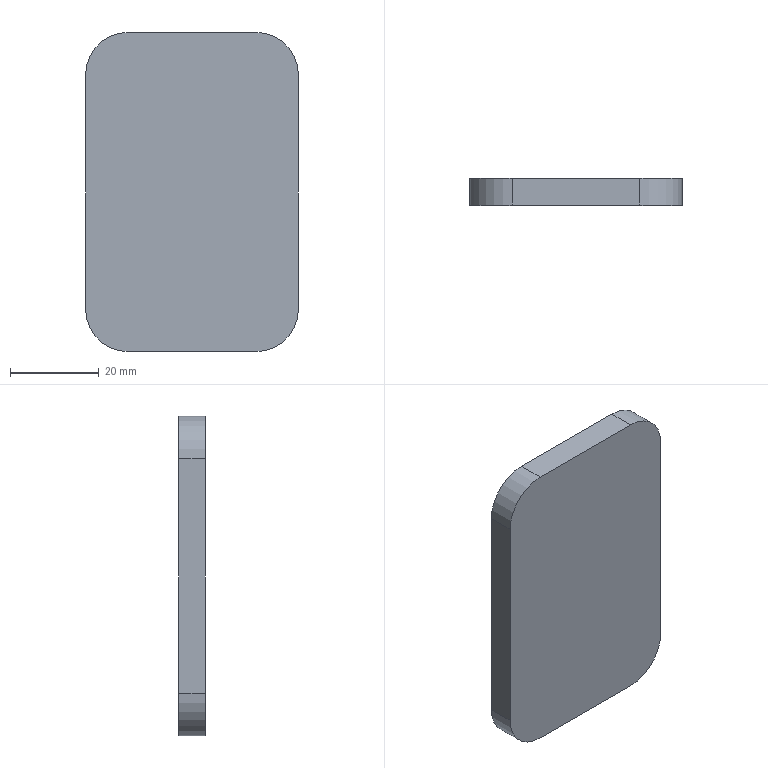Part | NX | 1 solid | 10 faces | box 48 x 6 x 72 mm | volume 20261 mm3 | plane 6 | cylinder 4 | commonest cylinder face diameters 19.2 x4
STEP:
#1=CARTESIAN_POINT('',(-7.326,-756.819,634.353));
#2=VERTEX_POINT('',#1);
#3=CARTESIAN_POINT('',(-16.926,-756.819,643.953));
#4=VERTEX_POINT('',#3);
#5=CARTESIAN_POINT('',(-16.926,-756.819,634.353));
#6=DIRECTION('',(0.,-1.,0.));
#7=DIRECTION('',(0.,0.,-1.));
#8=AXIS2_PLACEMENT_3D('',#5,#6,#7);
#9=CIRCLE('',#8,9.6);
#10=EDGE_CURVE('',#2,#4,#9,.T.);
#11=ORIENTED_EDGE('',*,*,#10,.T.);
#12=CARTESIAN_POINT('',(-16.926,-762.819,643.953));
#13=VERTEX_POINT('',#12);
#14=CARTESIAN_POINT('',(-16.926,-762.819,643.953));
#15=DIRECTION('',(0.,1.,0.));
#16=VECTOR('',#15,1.);
#17=LINE('',#14,#16);
#18=EDGE_CURVE('',#13,#4,#17,.T.);
#19=ORIENTED_EDGE('',*,*,#18,.F.);
#20=CARTESIAN_POINT('',(-7.326,-762.819,634.353));
#21=VERTEX_POINT('',#20);
#22=CARTESIAN_POINT('',(-16.926,-762.819,634.353));
#23=DIRECTION('',(0.,-1.,0.));
#24=DIRECTION('',(0.,0.,-1.));
#25=AXIS2_PLACEMENT_3D('',#22,#23,#24);
#26=CIRCLE('',#25,9.6);
#27=EDGE_CURVE('',#21,#13,#26,.T.);
#28=ORIENTED_EDGE('',*,*,#27,.F.);
#29=CARTESIAN_POINT('',(-7.326,-762.819,634.353));
#30=DIRECTION('',(0.,1.,0.));
#31=VECTOR('',#30,1.);
#32=LINE('',#29,#31);
#33=EDGE_CURVE('',#21,#2,#32,.T.);
#34=ORIENTED_EDGE('',*,*,#33,.T.);
#35=EDGE_LOOP('',(#11,#19,#28,#34));
#36=FACE_OUTER_BOUND('',#35,.T.);
#37=CARTESIAN_POINT('',(-16.926,-762.819,634.353));
#38=DIRECTION('',(0.,1.,0.));
#39=DIRECTION('',(0.,0.,1.));
#40=AXIS2_PLACEMENT_3D('',#37,#38,#39);
#41=CYLINDRICAL_SURFACE('',#40,9.6);
#42=ADVANCED_FACE('',(#36),#41,.T.);
#43=CARTESIAN_POINT('',(-45.726,-756.819,643.953));
#44=VERTEX_POINT('',#43);
#45=CARTESIAN_POINT('',(-16.926,-756.819,643.953));
#46=DIRECTION('',(-1.,0.,0.));
#47=VECTOR('',#46,1.);
#48=LINE('',#45,#47);
#49=EDGE_CURVE('',#4,#44,#48,.T.);
#50=ORIENTED_EDGE('',*,*,#49,.T.);
#51=CARTESIAN_POINT('',(-45.726,-762.819,643.953));
#52=VERTEX_POINT('',#51);
#53=CARTESIAN_POINT('',(-45.726,-762.819,643.953));
#54=DIRECTION('',(0.,1.,0.));
#55=VECTOR('',#54,1.);
#56=LINE('',#53,#55);
#57=EDGE_CURVE('',#52,#44,#56,.T.);
#58=ORIENTED_EDGE('',*,*,#57,.F.);
#59=CARTESIAN_POINT('',(-16.926,-762.819,643.953));
#60=DIRECTION('',(-1.,0.,0.));
#61=VECTOR('',#60,1.);
#62=LINE('',#59,#61);
#63=EDGE_CURVE('',#13,#52,#62,.T.);
#64=ORIENTED_EDGE('',*,*,#63,.F.);
#65=ORIENTED_EDGE('',*,*,#18,.T.);
#66=EDGE_LOOP('',(#50,#58,#64,#65));
#67=FACE_OUTER_BOUND('',#66,.T.);
#68=CARTESIAN_POINT('',(-16.926,-762.819,643.953));
#69=DIRECTION('',(0.,0.,-1.));
#70=DIRECTION('',(-1.,0.,0.));
#71=AXIS2_PLACEMENT_3D('',#68,#69,#70);
#72=PLANE('',#71);
#73=ADVANCED_FACE('',(#67),#72,.F.);
#74=CARTESIAN_POINT('',(-55.326,-756.819,634.353));
#75=VERTEX_POINT('',#74);
#76=CARTESIAN_POINT('',(-45.726,-756.819,634.353));
#77=DIRECTION('',(0.,-1.,0.));
#78=DIRECTION('',(0.,0.,-1.));
#79=AXIS2_PLACEMENT_3D('',#76,#77,#78);
#80=CIRCLE('',#79,9.6);
#81=EDGE_CURVE('',#44,#75,#80,.T.);
#82=ORIENTED_EDGE('',*,*,#81,.T.);
#83=CARTESIAN_POINT('',(-55.326,-762.819,634.353));
#84=VERTEX_POINT('',#83);
#85=CARTESIAN_POINT('',(-55.326,-762.819,634.353));
#86=DIRECTION('',(0.,1.,0.));
#87=VECTOR('',#86,1.);
#88=LINE('',#85,#87);
#89=EDGE_CURVE('',#84,#75,#88,.T.);
#90=ORIENTED_EDGE('',*,*,#89,.F.);
#91=CARTESIAN_POINT('',(-45.726,-762.819,634.353));
#92=DIRECTION('',(0.,-1.,0.));
#93=DIRECTION('',(0.,0.,-1.));
#94=AXIS2_PLACEMENT_3D('',#91,#92,#93);
#95=CIRCLE('',#94,9.6);
#96=EDGE_CURVE('',#52,#84,#95,.T.);
#97=ORIENTED_EDGE('',*,*,#96,.F.);
#98=ORIENTED_EDGE('',*,*,#57,.T.);
#99=EDGE_LOOP('',(#82,#90,#97,#98));
#100=FACE_OUTER_BOUND('',#99,.T.);
#101=CARTESIAN_POINT('',(-45.726,-762.819,634.353));
#102=DIRECTION('',(0.,1.,0.));
#103=DIRECTION('',(0.,0.,1.));
#104=AXIS2_PLACEMENT_3D('',#101,#102,#103);
#105=CYLINDRICAL_SURFACE('',#104,9.6);
#106=ADVANCED_FACE('',(#100),#105,.T.);
#107=CARTESIAN_POINT('',(-55.326,-756.819,581.553));
#108=VERTEX_POINT('',#107);
#109=CARTESIAN_POINT('',(-55.326,-756.819,634.353));
#110=DIRECTION('',(0.,0.,-1.));
#111=VECTOR('',#110,1.);
#112=LINE('',#109,#111);
#113=EDGE_CURVE('',#75,#108,#112,.T.);
#114=ORIENTED_EDGE('',*,*,#113,.T.);
#115=CARTESIAN_POINT('',(-55.326,-762.819,581.553));
#116=VERTEX_POINT('',#115);
#117=CARTESIAN_POINT('',(-55.326,-762.819,581.553));
#118=DIRECTION('',(0.,1.,0.));
#119=VECTOR('',#118,1.);
#120=LINE('',#117,#119);
#121=EDGE_CURVE('',#116,#108,#120,.T.);
#122=ORIENTED_EDGE('',*,*,#121,.F.);
#123=CARTESIAN_POINT('',(-55.326,-762.819,634.353));
#124=DIRECTION('',(0.,0.,-1.));
#125=VECTOR('',#124,1.);
#126=LINE('',#123,#125);
#127=EDGE_CURVE('',#84,#116,#126,.T.);
#128=ORIENTED_EDGE('',*,*,#127,.F.);
#129=ORIENTED_EDGE('',*,*,#89,.T.);
#130=EDGE_LOOP('',(#114,#122,#128,#129));
#131=FACE_OUTER_BOUND('',#130,.T.);
#132=CARTESIAN_POINT('',(-55.326,-762.819,634.353));
#133=DIRECTION('',(1.,0.,0.));
#134=DIRECTION('',(0.,0.,-1.));
#135=AXIS2_PLACEMENT_3D('',#132,#133,#134);
#136=PLANE('',#135);
#137=ADVANCED_FACE('',(#131),#136,.F.);
#138=CARTESIAN_POINT('',(-45.726,-756.819,571.953));
#139=VERTEX_POINT('',#138);
#140=CARTESIAN_POINT('',(-45.726,-756.819,581.553));
#141=DIRECTION('',(0.,-1.,0.));
#142=DIRECTION('',(0.,0.,-1.));
#143=AXIS2_PLACEMENT_3D('',#140,#141,#142);
#144=CIRCLE('',#143,9.6);
#145=EDGE_CURVE('',#108,#139,#144,.T.);
#146=ORIENTED_EDGE('',*,*,#145,.T.);
#147=CARTESIAN_POINT('',(-45.726,-762.819,571.953));
#148=VERTEX_POINT('',#147);
#149=CARTESIAN_POINT('',(-45.726,-762.819,571.953));
#150=DIRECTION('',(0.,1.,0.));
#151=VECTOR('',#150,1.);
#152=LINE('',#149,#151);
#153=EDGE_CURVE('',#148,#139,#152,.T.);
#154=ORIENTED_EDGE('',*,*,#153,.F.);
#155=CARTESIAN_POINT('',(-45.726,-762.819,581.553));
#156=DIRECTION('',(0.,-1.,0.));
#157=DIRECTION('',(0.,0.,-1.));
#158=AXIS2_PLACEMENT_3D('',#155,#156,#157);
#159=CIRCLE('',#158,9.6);
#160=EDGE_CURVE('',#116,#148,#159,.T.);
#161=ORIENTED_EDGE('',*,*,#160,.F.);
#162=ORIENTED_EDGE('',*,*,#121,.T.);
#163=EDGE_LOOP('',(#146,#154,#161,#162));
#164=FACE_OUTER_BOUND('',#163,.T.);
#165=CARTESIAN_POINT('',(-45.726,-762.819,581.553));
#166=DIRECTION('',(0.,1.,0.));
#167=DIRECTION('',(0.,0.,1.));
#168=AXIS2_PLACEMENT_3D('',#165,#166,#167);
#169=CYLINDRICAL_SURFACE('',#168,9.6);
#170=ADVANCED_FACE('',(#164),#169,.T.);
#171=CARTESIAN_POINT('',(-16.926,-756.819,571.953));
#172=VERTEX_POINT('',#171);
#173=CARTESIAN_POINT('',(-45.726,-756.819,571.953));
#174=DIRECTION('',(1.,0.,0.));
#175=VECTOR('',#174,1.);
#176=LINE('',#173,#175);
#177=EDGE_CURVE('',#139,#172,#176,.T.);
#178=ORIENTED_EDGE('',*,*,#177,.T.);
#179=CARTESIAN_POINT('',(-16.926,-762.819,571.953));
#180=VERTEX_POINT('',#179);
#181=CARTESIAN_POINT('',(-16.926,-762.819,571.953));
#182=DIRECTION('',(0.,1.,0.));
#183=VECTOR('',#182,1.);
#184=LINE('',#181,#183);
#185=EDGE_CURVE('',#180,#172,#184,.T.);
#186=ORIENTED_EDGE('',*,*,#185,.F.);
#187=CARTESIAN_POINT('',(-45.726,-762.819,571.953));
#188=DIRECTION('',(1.,0.,0.));
#189=VECTOR('',#188,1.);
#190=LINE('',#187,#189);
#191=EDGE_CURVE('',#148,#180,#190,.T.);
#192=ORIENTED_EDGE('',*,*,#191,.F.);
#193=ORIENTED_EDGE('',*,*,#153,.T.);
#194=EDGE_LOOP('',(#178,#186,#192,#193));
#195=FACE_OUTER_BOUND('',#194,.T.);
#196=CARTESIAN_POINT('',(-45.726,-762.819,571.953));
#197=DIRECTION('',(0.,0.,1.));
#198=DIRECTION('',(1.,0.,0.));
#199=AXIS2_PLACEMENT_3D('',#196,#197,#198);
#200=PLANE('',#199);
#201=ADVANCED_FACE('',(#195),#200,.F.);
#202=CARTESIAN_POINT('',(-7.326,-756.819,581.553));
#203=VERTEX_POINT('',#202);
#204=CARTESIAN_POINT('',(-16.926,-756.819,581.553));
#205=DIRECTION('',(0.,-1.,0.));
#206=DIRECTION('',(0.,0.,-1.));
#207=AXIS2_PLACEMENT_3D('',#204,#205,#206);
#208=CIRCLE('',#207,9.6);
#209=EDGE_CURVE('',#172,#203,#208,.T.);
#210=ORIENTED_EDGE('',*,*,#209,.T.);
#211=CARTESIAN_POINT('',(-7.326,-762.819,581.553));
#212=VERTEX_POINT('',#211);
#213=CARTESIAN_POINT('',(-7.326,-762.819,581.553));
#214=DIRECTION('',(0.,1.,0.));
#215=VECTOR('',#214,1.);
#216=LINE('',#213,#215);
#217=EDGE_CURVE('',#212,#203,#216,.T.);
#218=ORIENTED_EDGE('',*,*,#217,.F.);
#219=CARTESIAN_POINT('',(-16.926,-762.819,581.553));
#220=DIRECTION('',(0.,-1.,0.));
#221=DIRECTION('',(0.,0.,-1.));
#222=AXIS2_PLACEMENT_3D('',#219,#220,#221);
#223=CIRCLE('',#222,9.6);
#224=EDGE_CURVE('',#180,#212,#223,.T.);
#225=ORIENTED_EDGE('',*,*,#224,.F.);
#226=ORIENTED_EDGE('',*,*,#185,.T.);
#227=EDGE_LOOP('',(#210,#218,#225,#226));
#228=FACE_OUTER_BOUND('',#227,.T.);
#229=CARTESIAN_POINT('',(-16.926,-762.819,581.553));
#230=DIRECTION('',(0.,1.,0.));
#231=DIRECTION('',(0.,0.,1.));
#232=AXIS2_PLACEMENT_3D('',#229,#230,#231);
#233=CYLINDRICAL_SURFACE('',#232,9.6);
#234=ADVANCED_FACE('',(#228),#233,.T.);
#235=CARTESIAN_POINT('',(-7.326,-756.819,581.553));
#236=DIRECTION('',(0.,0.,1.));
#237=VECTOR('',#236,1.);
#238=LINE('',#235,#237);
#239=EDGE_CURVE('',#203,#2,#238,.T.);
#240=ORIENTED_EDGE('',*,*,#239,.T.);
#241=ORIENTED_EDGE('',*,*,#33,.F.);
#242=CARTESIAN_POINT('',(-7.326,-762.819,581.553));
#243=DIRECTION('',(0.,0.,1.));
#244=VECTOR('',#243,1.);
#245=LINE('',#242,#244);
#246=EDGE_CURVE('',#212,#21,#245,.T.);
#247=ORIENTED_EDGE('',*,*,#246,.F.);
#248=ORIENTED_EDGE('',*,*,#217,.T.);
#249=EDGE_LOOP('',(#240,#241,#247,#248));
#250=FACE_OUTER_BOUND('',#249,.T.);
#251=CARTESIAN_POINT('',(-7.326,-762.819,581.553));
#252=DIRECTION('',(-1.,0.,0.));
#253=DIRECTION('',(0.,0.,1.));
#254=AXIS2_PLACEMENT_3D('',#251,#252,#253);
#255=PLANE('',#254);
#256=ADVANCED_FACE('',(#250),#255,.F.);
#257=ORIENTED_EDGE('',*,*,#27,.T.);
#258=ORIENTED_EDGE('',*,*,#63,.T.);
#259=ORIENTED_EDGE('',*,*,#96,.T.);
#260=ORIENTED_EDGE('',*,*,#127,.T.);
#261=ORIENTED_EDGE('',*,*,#160,.T.);
#262=ORIENTED_EDGE('',*,*,#191,.T.);
#263=ORIENTED_EDGE('',*,*,#224,.T.);
#264=ORIENTED_EDGE('',*,*,#246,.T.);
#265=EDGE_LOOP('',(#257,#258,#259,#260,#261,#262,#263,#264));
#266=FACE_OUTER_BOUND('',#265,.T.);
#267=CARTESIAN_POINT('',(-16.926,-762.819,634.353));
#268=DIRECTION('',(0.,-1.,0.));
#269=DIRECTION('',(0.,0.,-1.));
#270=AXIS2_PLACEMENT_3D('',#267,#268,#269);
#271=PLANE('',#270);
#272=ADVANCED_FACE('',(#266),#271,.T.);
#273=ORIENTED_EDGE('',*,*,#10,.F.);
#274=ORIENTED_EDGE('',*,*,#239,.F.);
#275=ORIENTED_EDGE('',*,*,#209,.F.);
#276=ORIENTED_EDGE('',*,*,#177,.F.);
#277=ORIENTED_EDGE('',*,*,#145,.F.);
#278=ORIENTED_EDGE('',*,*,#113,.F.);
#279=ORIENTED_EDGE('',*,*,#81,.F.);
#280=ORIENTED_EDGE('',*,*,#49,.F.);
#281=EDGE_LOOP('',(#273,#274,#275,#276,#277,#278,#279,#280));
#282=FACE_OUTER_BOUND('',#281,.T.);
#283=CARTESIAN_POINT('',(-16.926,-756.819,634.353));
#284=DIRECTION('',(0.,-1.,0.));
#285=DIRECTION('',(0.,0.,-1.));
#286=AXIS2_PLACEMENT_3D('',#283,#284,#285);
#287=PLANE('',#286);
#288=ADVANCED_FACE('',(#282),#287,.F.);
#289=CLOSED_SHELL('',(#42,#73,#106,#137,#170,#201,#234,#256,#272,#288));
#290=MANIFOLD_SOLID_BREP('',#289);
#291=(LENGTH_UNIT()NAMED_UNIT(*)SI_UNIT(.MILLI.,.METRE.));
#292=UNCERTAINTY_MEASURE_WITH_UNIT(LENGTH_MEASURE(0.00002),#291,'','');
#293=(NAMED_UNIT(*)PLANE_ANGLE_UNIT()SI_UNIT($,.RADIAN.));
#294=PLANE_ANGLE_MEASURE_WITH_UNIT(PLANE_ANGLE_MEASURE(0.01745),#293);
#295=DIMENSIONAL_EXPONENTS(0.,0.,0.,0.,0.,0.,0.);
#296=(CONVERSION_BASED_UNIT('DEGREE',#294)NAMED_UNIT(#295)PLANE_ANGLE_UNIT());
#297=(NAMED_UNIT(*)SI_UNIT($,.STERADIAN.)SOLID_ANGLE_UNIT());
#298=(GEOMETRIC_REPRESENTATION_CONTEXT(3)GLOBAL_UNCERTAINTY_ASSIGNED_CONTEXT((#292))GLOBAL_UNIT_ASSIGNED_CONTEXT((#291,#296,#297))REPRESENTATION_CONTEXT('',''));
#299=ADVANCED_BREP_SHAPE_REPRESENTATION('',(#290),#298);